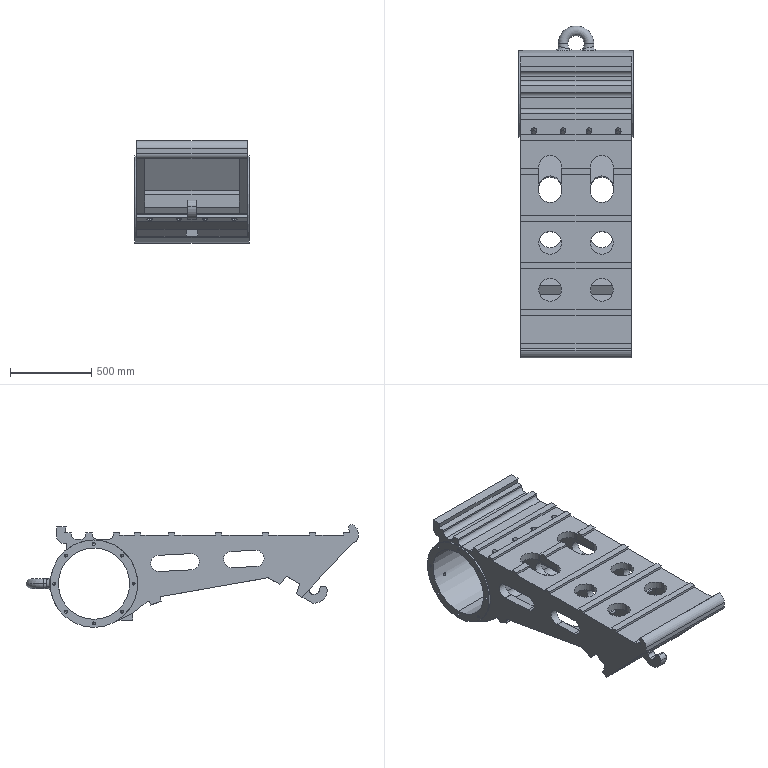Part | SolidWorks | features ICE 12, MirrorPattern 5, 3DProfileFeature 4, HoleWzd 4, Fillet 2, CirPattern 1, Extrusion 1, Revolution 1 | 2 solids | 299 faces | box 704 x 2050 x 634.865 mm | volume 188123623 mm3 | cylinder 129 | plane 124 | cone 36 | torus 6 | spline 4 | commonest cylinder face diameters 17.5 x40 100 x19 140 x18 36 x16 12 x6 80 x6